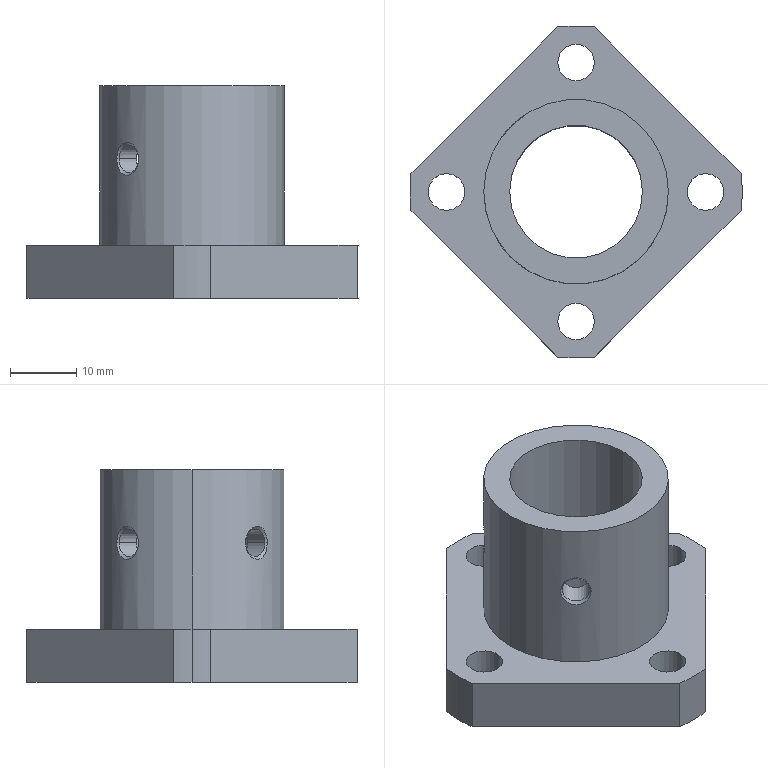Part | SolidWorks | features BaseBody 1 | 1 solid | 32 faces | box 50 x 50 x 32 mm | volume 15595 mm3 | cylinder 21 | plane 7 | cone 4 | commonest cylinder face diameters 5.5 x8 50 x5 4.134 x4 20 x2 27.8 x2
STEP:
#1=CARTESIAN_POINT('',(-11.324,8.061,13.));
#2=VERTEX_POINT('',#1);
#3=CARTESIAN_POINT('',(-8.061,11.324,13.));
#4=VERTEX_POINT('',#3);
#5=CARTESIAN_POINT('',(-11.324,8.061,13.));
#6=CARTESIAN_POINT('',(-11.324,8.061,12.686));
#7=CARTESIAN_POINT('',(-11.291,8.108,12.369));
#8=CARTESIAN_POINT('',(-11.194,8.241,11.927));
#9=CARTESIAN_POINT('',(-11.153,8.296,11.784));
#10=CARTESIAN_POINT('',(-11.055,8.426,11.513));
#11=CARTESIAN_POINT('',(-10.998,8.5,11.386));
#12=CARTESIAN_POINT('',(-10.869,8.666,11.151));
#13=CARTESIAN_POINT('',(-10.795,8.757,11.042));
#14=CARTESIAN_POINT('',(-10.635,8.952,10.853));
#15=CARTESIAN_POINT('',(-10.547,9.055,10.772));
#16=CARTESIAN_POINT('',(-10.357,9.271,10.637));
#17=CARTESIAN_POINT('',(-10.257,9.382,10.586));
#18=CARTESIAN_POINT('',(-10.048,9.606,10.517));
#19=CARTESIAN_POINT('',(-9.936,9.721,10.5));
#20=CARTESIAN_POINT('',(-9.603,10.054,10.501));
#21=CARTESIAN_POINT('',(-9.371,10.27,10.574));
#22=CARTESIAN_POINT('',(-9.052,10.55,10.774));
#23=CARTESIAN_POINT('',(-8.948,10.638,10.857));
#24=CARTESIAN_POINT('',(-8.753,10.799,11.047));
#25=CARTESIAN_POINT('',(-8.663,10.87,11.154));
#26=CARTESIAN_POINT('',(-8.499,10.999,11.388));
#27=CARTESIAN_POINT('',(-8.424,11.057,11.517));
#28=CARTESIAN_POINT('',(-8.295,11.154,11.787));
#29=CARTESIAN_POINT('',(-8.24,11.194,11.928));
#30=CARTESIAN_POINT('',(-8.152,11.259,12.222));
#31=CARTESIAN_POINT('',(-8.117,11.284,12.377));
#32=CARTESIAN_POINT('',(-8.072,11.316,12.686));
#33=CARTESIAN_POINT('',(-8.061,11.324,12.843));
#34=CARTESIAN_POINT('',(-8.061,11.324,13.));
#35=B_SPLINE_CURVE_WITH_KNOTS('',3,(#5,#6,#7,#8,#9,#10,#11,#12,#13,#14,#15,#16,#17,#18,#19,#20,#21,#22,#23,#24,#25,#26,#27,#28,#29,#30,#31,#32,#33,#34),.UNSPECIFIED.,.F.,.F.,(4,2,2,2,2,2,2,2,2,2,2,2,2,2,4),(0.003537,0.004487,0.004962,0.005436,0.005911,0.006386,0.006861,0.007336,0.008285,0.00876,0.009235,0.009709,0.01018,0.01066,0.01113),.UNSPECIFIED.);
#36=EDGE_CURVE('',#2,#4,#35,.T.);
#37=ORIENTED_EDGE('',*,*,#36,.T.);
#38=CARTESIAN_POINT('',(-8.061,11.324,13.));
#39=CARTESIAN_POINT('',(-8.061,11.324,13.157));
#40=CARTESIAN_POINT('',(-8.073,11.316,13.317));
#41=CARTESIAN_POINT('',(-8.118,11.283,13.626));
#42=CARTESIAN_POINT('',(-8.152,11.259,13.777));
#43=CARTESIAN_POINT('',(-8.285,11.161,14.221));
#44=CARTESIAN_POINT('',(-8.417,11.064,14.495));
#45=CARTESIAN_POINT('',(-8.666,10.869,14.849));
#46=CARTESIAN_POINT('',(-8.756,10.796,14.956));
#47=CARTESIAN_POINT('',(-8.95,10.636,15.145));
#48=CARTESIAN_POINT('',(-9.054,10.547,15.228));
#49=CARTESIAN_POINT('',(-9.376,10.266,15.428));
#50=CARTESIAN_POINT('',(-9.607,10.051,15.5));
#51=CARTESIAN_POINT('',(-10.051,9.607,15.5));
#52=CARTESIAN_POINT('',(-10.269,9.372,15.427));
#53=CARTESIAN_POINT('',(-10.55,9.051,15.226));
#54=CARTESIAN_POINT('',(-10.637,8.949,15.144));
#55=CARTESIAN_POINT('',(-10.797,8.755,14.955));
#56=CARTESIAN_POINT('',(-10.871,8.663,14.846));
#57=CARTESIAN_POINT('',(-10.999,8.499,14.612));
#58=CARTESIAN_POINT('',(-11.056,8.425,14.486));
#59=CARTESIAN_POINT('',(-11.153,8.296,14.215));
#60=CARTESIAN_POINT('',(-11.194,8.24,14.071));
#61=CARTESIAN_POINT('',(-11.259,8.152,13.778));
#62=CARTESIAN_POINT('',(-11.283,8.118,13.626));
#63=CARTESIAN_POINT('',(-11.316,8.072,13.315));
#64=CARTESIAN_POINT('',(-11.324,8.061,13.157));
#65=CARTESIAN_POINT('',(-11.324,8.061,13.));
#66=B_SPLINE_CURVE_WITH_KNOTS('',3,(#38,#39,#40,#41,#42,#43,#44,#45,#46,#47,#48,#49,#50,#51,#52,#53,#54,#55,#56,#57,#58,#59,#60,#61,#62,#63,#64,#65),.UNSPECIFIED.,.F.,.F.,(4,2,2,2,2,2,2,2,2,2,2,2,2,4),(0.01113,0.01161,0.01208,0.01303,0.01351,0.01398,0.01493,0.01588,0.01635,0.01683,0.0173,0.01778,0.01825,0.01873),.UNSPECIFIED.);
#67=EDGE_CURVE('',#4,#2,#66,.T.);
#68=ORIENTED_EDGE('',*,*,#67,.T.);
#69=EDGE_LOOP('',(#37,#68));
#70=FACE_BOUND('',#69,.T.);
#71=CARTESIAN_POINT('',(-13.9,0.,24.));
#72=VERTEX_POINT('',#71);
#73=CARTESIAN_POINT('',(13.9,0.,24.));
#74=VERTEX_POINT('',#73);
#75=CARTESIAN_POINT('',(0.,0.,24.));
#76=DIRECTION('',(0.,0.,-1.));
#77=DIRECTION('',(-1.,0.,0.));
#78=AXIS2_PLACEMENT_3D('',#75,#76,#77);
#79=CIRCLE('',#78,13.9);
#80=EDGE_CURVE('',#72,#74,#79,.T.);
#81=ORIENTED_EDGE('',*,*,#80,.T.);
#82=CARTESIAN_POINT('',(13.9,0.,0.));
#83=VERTEX_POINT('',#82);
#84=CARTESIAN_POINT('',(13.9,0.,0.));
#85=DIRECTION('',(0.,0.,-1.));
#86=VECTOR('',#85,1000.);
#87=LINE('',#84,#86);
#88=EDGE_CURVE('',#74,#83,#87,.T.);
#89=ORIENTED_EDGE('',*,*,#88,.T.);
#90=CARTESIAN_POINT('',(-13.9,0.,0.));
#91=VERTEX_POINT('',#90);
#92=CARTESIAN_POINT('',(0.,0.,0.));
#93=DIRECTION('',(0.,0.,1.));
#94=DIRECTION('',(-1.,0.,0.));
#95=AXIS2_PLACEMENT_3D('',#92,#93,#94);
#96=CIRCLE('',#95,13.9);
#97=EDGE_CURVE('',#83,#91,#96,.T.);
#98=ORIENTED_EDGE('',*,*,#97,.T.);
#99=CARTESIAN_POINT('',(-13.9,0.,0.));
#100=DIRECTION('',(0.,0.,-1.));
#101=VECTOR('',#100,1000.);
#102=LINE('',#99,#101);
#103=EDGE_CURVE('',#72,#91,#102,.T.);
#104=ORIENTED_EDGE('',*,*,#103,.F.);
#105=EDGE_LOOP('',(#81,#89,#98,#104));
#106=FACE_OUTER_BOUND('',#105,.T.);
#107=CARTESIAN_POINT('',(0.,0.,0.));
#108=DIRECTION('',(0.,0.,-1.));
#109=DIRECTION('',(-1.,0.,0.));
#110=AXIS2_PLACEMENT_3D('',#107,#108,#109);
#111=CYLINDRICAL_SURFACE('',#110,13.9);
#112=ADVANCED_FACE('',(#70,#106),#111,.T.);
#113=CARTESIAN_POINT('',(-25.,0.,0.));
#114=VERTEX_POINT('',#113);
#115=CARTESIAN_POINT('',(-24.851,-2.726,0.));
#116=VERTEX_POINT('',#115);
#117=CARTESIAN_POINT('',(0.,0.,0.));
#118=DIRECTION('',(0.,0.,1.));
#119=DIRECTION('',(-1.,0.,0.));
#120=AXIS2_PLACEMENT_3D('',#117,#118,#119);
#121=CIRCLE('',#120,25.);
#122=EDGE_CURVE('',#114,#116,#121,.T.);
#123=ORIENTED_EDGE('',*,*,#122,.F.);
#124=CARTESIAN_POINT('',(-25.,0.,-8.));
#125=VERTEX_POINT('',#124);
#126=CARTESIAN_POINT('',(-25.,0.,0.));
#127=DIRECTION('',(0.,0.,-1.));
#128=VECTOR('',#127,1000.);
#129=LINE('',#126,#128);
#130=EDGE_CURVE('',#114,#125,#129,.T.);
#131=ORIENTED_EDGE('',*,*,#130,.T.);
#132=CARTESIAN_POINT('',(-24.851,-2.726,-8.));
#133=VERTEX_POINT('',#132);
#134=CARTESIAN_POINT('',(0.,0.,-8.));
#135=DIRECTION('',(0.,0.,1.));
#136=DIRECTION('',(-1.,0.,0.));
#137=AXIS2_PLACEMENT_3D('',#134,#135,#136);
#138=CIRCLE('',#137,25.);
#139=EDGE_CURVE('',#125,#133,#138,.T.);
#140=ORIENTED_EDGE('',*,*,#139,.T.);
#141=CARTESIAN_POINT('',(-24.851,-2.726,-8.));
#142=DIRECTION('',(0.,0.,-1.));
#143=VECTOR('',#142,1000.);
#144=LINE('',#141,#143);
#145=EDGE_CURVE('',#116,#133,#144,.T.);
#146=ORIENTED_EDGE('',*,*,#145,.F.);
#147=EDGE_LOOP('',(#123,#131,#140,#146));
#148=FACE_OUTER_BOUND('',#147,.T.);
#149=CARTESIAN_POINT('',(0.,0.,0.));
#150=DIRECTION('',(0.,0.,-1.));
#151=DIRECTION('',(-1.,0.,0.));
#152=AXIS2_PLACEMENT_3D('',#149,#150,#151);
#153=CYLINDRICAL_SURFACE('',#152,25.);
#154=ADVANCED_FACE('',(#148),#153,.T.);
#155=CARTESIAN_POINT('',(-16.75,0.,0.));
#156=VERTEX_POINT('',#155);
#157=CARTESIAN_POINT('',(-22.25,0.,0.));
#158=VERTEX_POINT('',#157);
#159=CARTESIAN_POINT('',(-19.5,0.,0.));
#160=DIRECTION('',(0.,0.,-1.));
#161=DIRECTION('',(-1.,0.,0.));
#162=AXIS2_PLACEMENT_3D('',#159,#160,#161);
#163=CIRCLE('',#162,2.75);
#164=EDGE_CURVE('',#156,#158,#163,.T.);
#165=ORIENTED_EDGE('',*,*,#164,.F.);
#166=CARTESIAN_POINT('',(-16.75,0.,-8.));
#167=VERTEX_POINT('',#166);
#168=CARTESIAN_POINT('',(-16.75,0.,-8.));
#169=DIRECTION('',(0.,0.,-1.));
#170=VECTOR('',#169,1000.);
#171=LINE('',#168,#170);
#172=EDGE_CURVE('',#156,#167,#171,.T.);
#173=ORIENTED_EDGE('',*,*,#172,.T.);
#174=CARTESIAN_POINT('',(-22.25,0.,-8.));
#175=VERTEX_POINT('',#174);
#176=CARTESIAN_POINT('',(-19.5,0.,-8.));
#177=DIRECTION('',(0.,0.,1.));
#178=DIRECTION('',(-1.,0.,0.));
#179=AXIS2_PLACEMENT_3D('',#176,#177,#178);
#180=CIRCLE('',#179,2.75);
#181=EDGE_CURVE('',#175,#167,#180,.T.);
#182=ORIENTED_EDGE('',*,*,#181,.F.);
#183=CARTESIAN_POINT('',(-22.25,0.,-8.));
#184=DIRECTION('',(0.,0.,-1.));
#185=VECTOR('',#184,1000.);
#186=LINE('',#183,#185);
#187=EDGE_CURVE('',#158,#175,#186,.T.);
#188=ORIENTED_EDGE('',*,*,#187,.F.);
#189=EDGE_LOOP('',(#165,#173,#182,#188));
#190=FACE_OUTER_BOUND('',#189,.T.);
#191=CARTESIAN_POINT('',(-19.5,0.,-8.));
#192=DIRECTION('',(0.,0.,-1.));
#193=DIRECTION('',(-1.,0.,0.));
#194=AXIS2_PLACEMENT_3D('',#191,#192,#193);
#195=CYLINDRICAL_SURFACE('',#194,2.75);
#196=ADVANCED_FACE('',(#190),#195,.F.);
#197=CARTESIAN_POINT('',(2.75,-19.5,0.));
#198=VERTEX_POINT('',#197);
#199=CARTESIAN_POINT('',(-2.75,-19.5,0.));
#200=VERTEX_POINT('',#199);
#201=CARTESIAN_POINT('',(0.,-19.5,0.));
#202=DIRECTION('',(0.,0.,-1.));
#203=DIRECTION('',(-1.,0.,0.));
#204=AXIS2_PLACEMENT_3D('',#201,#202,#203);
#205=CIRCLE('',#204,2.75);
#206=EDGE_CURVE('',#198,#200,#205,.T.);
#207=ORIENTED_EDGE('',*,*,#206,.F.);
#208=CARTESIAN_POINT('',(2.75,-19.5,-8.));
#209=VERTEX_POINT('',#208);
#210=CARTESIAN_POINT('',(2.75,-19.5,-8.));
#211=DIRECTION('',(0.,0.,-1.));
#212=VECTOR('',#211,1000.);
#213=LINE('',#210,#212);
#214=EDGE_CURVE('',#198,#209,#213,.T.);
#215=ORIENTED_EDGE('',*,*,#214,.T.);
#216=CARTESIAN_POINT('',(-2.75,-19.5,-8.));
#217=VERTEX_POINT('',#216);
#218=CARTESIAN_POINT('',(0.,-19.5,-8.));
#219=DIRECTION('',(0.,0.,1.));
#220=DIRECTION('',(-1.,0.,0.));
#221=AXIS2_PLACEMENT_3D('',#218,#219,#220);
#222=CIRCLE('',#221,2.75);
#223=EDGE_CURVE('',#217,#209,#222,.T.);
#224=ORIENTED_EDGE('',*,*,#223,.F.);
#225=CARTESIAN_POINT('',(-2.75,-19.5,-8.));
#226=DIRECTION('',(0.,0.,-1.));
#227=VECTOR('',#226,1000.);
#228=LINE('',#225,#227);
#229=EDGE_CURVE('',#200,#217,#228,.T.);
#230=ORIENTED_EDGE('',*,*,#229,.F.);
#231=EDGE_LOOP('',(#207,#215,#224,#230));
#232=FACE_OUTER_BOUND('',#231,.T.);
#233=CARTESIAN_POINT('',(0.,-19.5,-8.));
#234=DIRECTION('',(0.,0.,-1.));
#235=DIRECTION('',(-1.,0.,0.));
#236=AXIS2_PLACEMENT_3D('',#233,#234,#235);
#237=CYLINDRICAL_SURFACE('',#236,2.75);
#238=ADVANCED_FACE('',(#232),#237,.F.);
#239=CARTESIAN_POINT('',(22.25,0.,0.));
#240=VERTEX_POINT('',#239);
#241=CARTESIAN_POINT('',(16.75,0.,0.));
#242=VERTEX_POINT('',#241);
#243=CARTESIAN_POINT('',(19.5,0.,0.));
#244=DIRECTION('',(0.,0.,-1.));
#245=DIRECTION('',(-1.,0.,0.));
#246=AXIS2_PLACEMENT_3D('',#243,#244,#245);
#247=CIRCLE('',#246,2.75);
#248=EDGE_CURVE('',#240,#242,#247,.T.);
#249=ORIENTED_EDGE('',*,*,#248,.F.);
#250=CARTESIAN_POINT('',(22.25,0.,-8.));
#251=VERTEX_POINT('',#250);
#252=CARTESIAN_POINT('',(22.25,0.,-8.));
#253=DIRECTION('',(0.,0.,-1.));
#254=VECTOR('',#253,1000.);
#255=LINE('',#252,#254);
#256=EDGE_CURVE('',#240,#251,#255,.T.);
#257=ORIENTED_EDGE('',*,*,#256,.T.);
#258=CARTESIAN_POINT('',(16.75,0.,-8.));
#259=VERTEX_POINT('',#258);
#260=CARTESIAN_POINT('',(19.5,0.,-8.));
#261=DIRECTION('',(0.,0.,1.));
#262=DIRECTION('',(-1.,0.,0.));
#263=AXIS2_PLACEMENT_3D('',#260,#261,#262);
#264=CIRCLE('',#263,2.75);
#265=EDGE_CURVE('',#259,#251,#264,.T.);
#266=ORIENTED_EDGE('',*,*,#265,.F.);
#267=CARTESIAN_POINT('',(16.75,0.,-8.));
#268=DIRECTION('',(0.,0.,-1.));
#269=VECTOR('',#268,1000.);
#270=LINE('',#267,#269);
#271=EDGE_CURVE('',#242,#259,#270,.T.);
#272=ORIENTED_EDGE('',*,*,#271,.F.);
#273=EDGE_LOOP('',(#249,#257,#266,#272));
#274=FACE_OUTER_BOUND('',#273,.T.);
#275=CARTESIAN_POINT('',(19.5,0.,-8.));
#276=DIRECTION('',(0.,0.,-1.));
#277=DIRECTION('',(-1.,0.,0.));
#278=AXIS2_PLACEMENT_3D('',#275,#276,#277);
#279=CYLINDRICAL_SURFACE('',#278,2.75);
#280=ADVANCED_FACE('',(#274),#279,.F.);
#281=CARTESIAN_POINT('',(2.75,19.5,0.));
#282=VERTEX_POINT('',#281);
#283=CARTESIAN_POINT('',(-2.75,19.5,0.));
#284=VERTEX_POINT('',#283);
#285=CARTESIAN_POINT('',(0.,19.5,0.));
#286=DIRECTION('',(0.,0.,-1.));
#287=DIRECTION('',(-1.,0.,0.));
#288=AXIS2_PLACEMENT_3D('',#285,#286,#287);
#289=CIRCLE('',#288,2.75);
#290=EDGE_CURVE('',#282,#284,#289,.T.);
#291=ORIENTED_EDGE('',*,*,#290,.F.);
#292=CARTESIAN_POINT('',(2.75,19.5,-8.));
#293=VERTEX_POINT('',#292);
#294=CARTESIAN_POINT('',(2.75,19.5,-8.));
#295=DIRECTION('',(0.,0.,-1.));
#296=VECTOR('',#295,1000.);
#297=LINE('',#294,#296);
#298=EDGE_CURVE('',#282,#293,#297,.T.);
#299=ORIENTED_EDGE('',*,*,#298,.T.);
#300=CARTESIAN_POINT('',(-2.75,19.5,-8.));
#301=VERTEX_POINT('',#300);
#302=CARTESIAN_POINT('',(0.,19.5,-8.));
#303=DIRECTION('',(0.,0.,1.));
#304=DIRECTION('',(-1.,0.,0.));
#305=AXIS2_PLACEMENT_3D('',#302,#303,#304);
#306=CIRCLE('',#305,2.75);
#307=EDGE_CURVE('',#301,#293,#306,.T.);
#308=ORIENTED_EDGE('',*,*,#307,.F.);
#309=CARTESIAN_POINT('',(-2.75,19.5,-8.));
#310=DIRECTION('',(0.,0.,-1.));
#311=VECTOR('',#310,1000.);
#312=LINE('',#309,#311);
#313=EDGE_CURVE('',#284,#301,#312,.T.);
#314=ORIENTED_EDGE('',*,*,#313,.F.);
#315=EDGE_LOOP('',(#291,#299,#308,#314));
#316=FACE_OUTER_BOUND('',#315,.T.);
#317=CARTESIAN_POINT('',(0.,19.5,-8.));
#318=DIRECTION('',(0.,0.,-1.));
#319=DIRECTION('',(-1.,0.,0.));
#320=AXIS2_PLACEMENT_3D('',#317,#318,#319);
#321=CYLINDRICAL_SURFACE('',#320,2.75);
#322=ADVANCED_FACE('',(#316),#321,.F.);
#323=CARTESIAN_POINT('',(-5.457,-8.38,13.));
#324=VERTEX_POINT('',#323);
#325=CARTESIAN_POINT('',(-8.38,-5.457,13.));
#326=VERTEX_POINT('',#325);
#327=CARTESIAN_POINT('',(-5.457,-8.38,13.));
#328=CARTESIAN_POINT('',(-5.457,-8.38,12.863));
#329=CARTESIAN_POINT('',(-5.468,-8.372,12.728));
#330=CARTESIAN_POINT('',(-5.513,-8.343,12.464));
#331=CARTESIAN_POINT('',(-5.547,-8.321,12.333));
#332=CARTESIAN_POINT('',(-5.635,-8.261,12.082));
#333=CARTESIAN_POINT('',(-5.688,-8.225,11.964));
#334=CARTESIAN_POINT('',(-5.813,-8.137,11.74));
#335=CARTESIAN_POINT('',(-5.884,-8.086,11.634));
#336=CARTESIAN_POINT('',(-6.039,-7.971,11.443));
#337=CARTESIAN_POINT('',(-6.122,-7.908,11.358));
#338=CARTESIAN_POINT('',(-6.3,-7.767,11.207));
#339=CARTESIAN_POINT('',(-6.393,-7.69,11.143));
#340=CARTESIAN_POINT('',(-6.678,-7.448,10.988));
#341=CARTESIAN_POINT('',(-6.879,-7.263,10.933));
#342=CARTESIAN_POINT('',(-7.166,-6.976,10.933));
#343=CARTESIAN_POINT('',(-7.261,-6.877,10.946));
#344=CARTESIAN_POINT('',(-7.441,-6.682,10.999));
#345=CARTESIAN_POINT('',(-7.527,-6.585,11.038));
#346=CARTESIAN_POINT('',(-7.689,-6.394,11.142));
#347=CARTESIAN_POINT('',(-7.766,-6.301,11.207));
#348=CARTESIAN_POINT('',(-7.906,-6.124,11.356));
#349=CARTESIAN_POINT('',(-7.97,-6.041,11.441));
#350=CARTESIAN_POINT('',(-8.086,-5.884,11.634));
#351=CARTESIAN_POINT('',(-8.137,-5.814,11.738));
#352=CARTESIAN_POINT('',(-8.225,-5.689,11.963));
#353=CARTESIAN_POINT('',(-8.262,-5.634,12.084));
#354=CARTESIAN_POINT('',(-8.35,-5.504,12.457));
#355=CARTESIAN_POINT('',(-8.38,-5.457,12.73));
#356=CARTESIAN_POINT('',(-8.38,-5.457,13.));
#357=B_SPLINE_CURVE_WITH_KNOTS('',3,(#327,#328,#329,#330,#331,#332,#333,#334,#335,#336,#337,#338,#339,#340,#341,#342,#343,#344,#345,#346,#347,#348,#349,#350,#351,#352,#353,#354,#355,#356),.UNSPECIFIED.,.F.,.F.,(4,2,2,2,2,2,2,2,2,2,2,2,2,2,4),(0.008144,0.008552,0.008959,0.009366,0.009774,0.01018,0.01059,0.0114,0.01181,0.01222,0.01262,0.01303,0.01344,0.01385,0.01466),.UNSPECIFIED.);
#358=EDGE_CURVE('',#324,#326,#357,.T.);
#359=ORIENTED_EDGE('',*,*,#358,.F.);
#360=CARTESIAN_POINT('',(-8.38,-5.457,13.));
#361=CARTESIAN_POINT('',(-8.38,-5.457,13.135));
#362=CARTESIAN_POINT('',(-8.372,-5.468,13.272));
#363=CARTESIAN_POINT('',(-8.343,-5.514,13.538));
#364=CARTESIAN_POINT('',(-8.321,-5.547,13.667));
#365=CARTESIAN_POINT('',(-8.262,-5.635,13.917));
#366=CARTESIAN_POINT('',(-8.224,-5.689,14.038));
#367=CARTESIAN_POINT('',(-8.137,-5.813,14.261));
#368=CARTESIAN_POINT('',(-8.087,-5.884,14.365));
#369=CARTESIAN_POINT('',(-7.913,-6.117,14.653));
#370=CARTESIAN_POINT('',(-7.772,-6.297,14.805));
#371=CARTESIAN_POINT('',(-7.527,-6.585,14.961));
#372=CARTESIAN_POINT('',(-7.441,-6.682,15.001));
#373=CARTESIAN_POINT('',(-7.261,-6.877,15.053));
#374=CARTESIAN_POINT('',(-7.166,-6.976,15.067));
#375=CARTESIAN_POINT('',(-6.975,-7.167,15.067));
#376=CARTESIAN_POINT('',(-6.878,-7.26,15.054));
#377=CARTESIAN_POINT('',(-6.682,-7.441,15.001));
#378=CARTESIAN_POINT('',(-6.583,-7.528,14.961));
#379=CARTESIAN_POINT('',(-6.299,-7.771,14.806));
#380=CARTESIAN_POINT('',(-6.116,-7.914,14.652));
#381=CARTESIAN_POINT('',(-5.885,-8.086,14.367));
#382=CARTESIAN_POINT('',(-5.813,-8.137,14.261));
#383=CARTESIAN_POINT('',(-5.688,-8.225,14.036));
#384=CARTESIAN_POINT('',(-5.635,-8.261,13.918));
#385=CARTESIAN_POINT('',(-5.547,-8.32,13.668));
#386=CARTESIAN_POINT('',(-5.513,-8.343,13.536));
#387=CARTESIAN_POINT('',(-5.468,-8.372,13.271));
#388=CARTESIAN_POINT('',(-5.457,-8.38,13.137));
#389=CARTESIAN_POINT('',(-5.457,-8.38,13.));
#390=B_SPLINE_CURVE_WITH_KNOTS('',3,(#360,#361,#362,#363,#364,#365,#366,#367,#368,#369,#370,#371,#372,#373,#374,#375,#376,#377,#378,#379,#380,#381,#382,#383,#384,#385,#386,#387,#388,#389),.UNSPECIFIED.,.F.,.F.,(4,2,2,2,2,2,2,2,2,2,2,2,2,2,4),(0.001626,0.002033,0.002441,0.002848,0.003255,0.00407,0.004478,0.004885,0.005293,0.0057,0.006515,0.006922,0.00733,0.007737,0.008144),.UNSPECIFIED.);
#391=EDGE_CURVE('',#326,#324,#390,.T.);
#392=ORIENTED_EDGE('',*,*,#391,.F.);
#393=EDGE_LOOP('',(#359,#392));
#394=FACE_BOUND('',#393,.T.);
#395=CARTESIAN_POINT('',(10.,0.,24.));
#396=VERTEX_POINT('',#395);
#397=CARTESIAN_POINT('',(-10.,0.,24.));
#398=VERTEX_POINT('',#397);
#399=CARTESIAN_POINT('',(0.,0.,24.));
#400=DIRECTION('',(0.,0.,-1.));
#401=DIRECTION('',(-1.,0.,0.));
#402=AXIS2_PLACEMENT_3D('',#399,#400,#401);
#403=CIRCLE('',#402,10.);
#404=EDGE_CURVE('',#396,#398,#403,.T.);
#405=ORIENTED_EDGE('',*,*,#404,.F.);
#406=CARTESIAN_POINT('',(10.,0.,-8.));
#407=VERTEX_POINT('',#406);
#408=CARTESIAN_POINT('',(10.,0.,0.));
#409=DIRECTION('',(0.,0.,-1.));
#410=VECTOR('',#409,1000.);
#411=LINE('',#408,#410);
#412=EDGE_CURVE('',#396,#407,#411,.T.);
#413=ORIENTED_EDGE('',*,*,#412,.T.);
#414=CARTESIAN_POINT('',(-10.,0.,-8.));
#415=VERTEX_POINT('',#414);
#416=CARTESIAN_POINT('',(0.,0.,-8.));
#417=DIRECTION('',(0.,0.,1.));
#418=DIRECTION('',(-1.,0.,0.));
#419=AXIS2_PLACEMENT_3D('',#416,#417,#418);
#420=CIRCLE('',#419,10.);
#421=EDGE_CURVE('',#415,#407,#420,.T.);
#422=ORIENTED_EDGE('',*,*,#421,.F.);
#423=CARTESIAN_POINT('',(-10.,0.,0.));
#424=DIRECTION('',(0.,0.,-1.));
#425=VECTOR('',#424,1000.);
#426=LINE('',#423,#425);
#427=EDGE_CURVE('',#398,#415,#426,.T.);
#428=ORIENTED_EDGE('',*,*,#427,.F.);
#429=EDGE_LOOP('',(#405,#413,#422,#428));
#430=FACE_OUTER_BOUND('',#429,.T.);
#431=CARTESIAN_POINT('',(0.,0.,0.));
#432=DIRECTION('',(0.,0.,-1.));
#433=DIRECTION('',(-1.,0.,0.));
#434=AXIS2_PLACEMENT_3D('',#431,#432,#433);
#435=CYLINDRICAL_SURFACE('',#434,10.);
#436=ADVANCED_FACE('',(#394,#430),#435,.F.);
#437=ORIENTED_EDGE('',*,*,#358,.T.);
#438=CARTESIAN_POINT('',(-10.984,-8.061,13.));
#439=VERTEX_POINT('',#438);
#440=CARTESIAN_POINT('',(-11.29,-8.367,13.));
#441=DIRECTION('',(-0.7071,-0.7071,0.));
#442=VECTOR('',#441,1000.);
#443=LINE('',#440,#442);
#444=EDGE_CURVE('',#326,#439,#443,.T.);
#445=ORIENTED_EDGE('',*,*,#444,.T.);
#446=CARTESIAN_POINT('',(-8.061,-10.984,13.));
#447=VERTEX_POINT('',#446);
#448=CARTESIAN_POINT('',(-9.523,-9.523,13.));
#449=DIRECTION('',(0.7071,0.7071,0.));
#450=DIRECTION('',(0.7071,-0.7071,0.));
#451=AXIS2_PLACEMENT_3D('',#448,#449,#450);
#452=CIRCLE('',#451,2.067);
#453=EDGE_CURVE('',#447,#439,#452,.T.);
#454=ORIENTED_EDGE('',*,*,#453,.F.);
#455=CARTESIAN_POINT('',(-8.367,-11.29,13.));
#456=DIRECTION('',(-0.7071,-0.7071,0.));
#457=VECTOR('',#456,1000.);
#458=LINE('',#455,#457);
#459=EDGE_CURVE('',#324,#447,#458,.T.);
#460=ORIENTED_EDGE('',*,*,#459,.F.);
#461=EDGE_LOOP('',(#437,#445,#454,#460));
#462=FACE_OUTER_BOUND('',#461,.T.);
#463=CARTESIAN_POINT('',(-9.829,-9.829,13.));
#464=DIRECTION('',(-0.7071,-0.7071,0.));
#465=DIRECTION('',(0.7071,-0.7071,0.));
#466=AXIS2_PLACEMENT_3D('',#463,#464,#465);
#467=CYLINDRICAL_SURFACE('',#466,2.067);
#468=ADVANCED_FACE('',(#462),#467,.F.);
#469=ORIENTED_EDGE('',*,*,#453,.T.);
#470=CARTESIAN_POINT('',(-11.324,-8.061,13.));
#471=VERTEX_POINT('',#470);
#472=CARTESIAN_POINT('',(-11.641,-8.061,13.));
#473=DIRECTION('',(-1.,0.,0.));
#474=VECTOR('',#473,1000.);
#475=LINE('',#472,#474);
#476=EDGE_CURVE('',#439,#471,#475,.T.);
#477=ORIENTED_EDGE('',*,*,#476,.T.);
#478=CARTESIAN_POINT('',(-8.061,-11.324,13.));
#479=VERTEX_POINT('',#478);
#480=CARTESIAN_POINT('',(-8.061,-11.324,13.));
#481=CARTESIAN_POINT('',(-8.061,-11.324,12.843));
#482=CARTESIAN_POINT('',(-8.072,-11.316,12.686));
#483=CARTESIAN_POINT('',(-8.118,-11.283,12.376));
#484=CARTESIAN_POINT('',(-8.152,-11.259,12.222));
#485=CARTESIAN_POINT('',(-8.285,-11.161,11.78));
#486=CARTESIAN_POINT('',(-8.418,-11.063,11.503));
#487=CARTESIAN_POINT('',(-8.665,-10.869,11.151));
#488=CARTESIAN_POINT('',(-8.757,-10.795,11.043));
#489=CARTESIAN_POINT('',(-8.952,-10.634,10.853));
#490=CARTESIAN_POINT('',(-9.054,-10.547,10.772));
#491=CARTESIAN_POINT('',(-9.27,-10.358,10.638));
#492=CARTESIAN_POINT('',(-9.382,-10.257,10.586));
#493=CARTESIAN_POINT('',(-9.606,-10.048,10.517));
#494=CARTESIAN_POINT('',(-9.72,-9.937,10.5));
#495=CARTESIAN_POINT('',(-9.944,-9.714,10.5));
#496=CARTESIAN_POINT('',(-10.052,-9.602,10.518));
#497=CARTESIAN_POINT('',(-10.262,-9.377,10.588));
#498=CARTESIAN_POINT('',(-10.363,-9.265,10.641));
#499=CARTESIAN_POINT('',(-10.643,-8.945,10.841));
#500=CARTESIAN_POINT('',(-10.806,-8.745,11.037));
#501=CARTESIAN_POINT('',(-11.064,-8.417,11.504));
#502=CARTESIAN_POINT('',(-11.162,-8.284,11.782));
#503=CARTESIAN_POINT('',(-11.291,-8.108,12.369));
#504=CARTESIAN_POINT('',(-11.324,-8.061,12.686));
#505=CARTESIAN_POINT('',(-11.324,-8.061,13.));
#506=B_SPLINE_CURVE_WITH_KNOTS('',3,(#480,#481,#482,#483,#484,#485,#486,#487,#488,#489,#490,#491,#492,#493,#494,#495,#496,#497,#498,#499,#500,#501,#502,#503,#504,#505),.UNSPECIFIED.,.F.,.F.,(4,2,2,2,2,2,2,2,2,2,2,2,4),(0.001887,0.002359,0.002831,0.003775,0.004246,0.004718,0.00519,0.005662,0.006134,0.006605,0.007549,0.008493,0.009436),.UNSPECIFIED.);
#507=EDGE_CURVE('',#479,#471,#506,.T.);
#508=ORIENTED_EDGE('',*,*,#507,.F.);
#509=CARTESIAN_POINT('',(-8.061,-11.641,13.));
#510=DIRECTION('',(0.,-1.,0.));
#511=VECTOR('',#510,1000.);
#512=LINE('',#509,#511);
#513=EDGE_CURVE('',#447,#479,#512,.T.);
#514=ORIENTED_EDGE('',*,*,#513,.F.);
#515=EDGE_LOOP('',(#469,#477,#508,#514));
#516=FACE_OUTER_BOUND('',#515,.T.);
#517=CARTESIAN_POINT('',(-9.851,-9.851,13.));
#518=DIRECTION('',(-0.7071,-0.7071,0.));
#519=DIRECTION('',(0.7071,-0.7071,0.));
#520=AXIS2_PLACEMENT_3D('',#517,#518,#519);
#521=CONICAL_SURFACE('',#520,2.532,0.7854);
#522=ADVANCED_FACE('',(#516),#521,.F.);
#523=CARTESIAN_POINT('',(-8.38,5.457,13.));
#524=VERTEX_POINT('',#523);
#525=CARTESIAN_POINT('',(-5.457,8.38,13.));
#526=VERTEX_POINT('',#525);
#527=CARTESIAN_POINT('',(-8.38,5.457,13.));
#528=CARTESIAN_POINT('',(-8.38,5.457,12.863));
#529=CARTESIAN_POINT('',(-8.372,5.468,12.728));
#530=CARTESIAN_POINT('',(-8.343,5.513,12.464));
#531=CARTESIAN_POINT('',(-8.321,5.547,12.333));
#532=CARTESIAN_POINT('',(-8.261,5.635,12.082));
#533=CARTESIAN_POINT('',(-8.225,5.688,11.964));
#534=CARTESIAN_POINT('',(-8.137,5.813,11.74));
#535=CARTESIAN_POINT('',(-8.086,5.884,11.634));
#536=CARTESIAN_POINT('',(-7.971,6.039,11.443));
#537=CARTESIAN_POINT('',(-7.908,6.122,11.358));
#538=CARTESIAN_POINT('',(-7.767,6.3,11.207));
#539=CARTESIAN_POINT('',(-7.69,6.393,11.143));
#540=CARTESIAN_POINT('',(-7.448,6.678,10.988));
#541=CARTESIAN_POINT('',(-7.263,6.879,10.933));
#542=CARTESIAN_POINT('',(-6.976,7.166,10.933));
#543=CARTESIAN_POINT('',(-6.877,7.261,10.946));
#544=CARTESIAN_POINT('',(-6.682,7.441,10.999));
#545=CARTESIAN_POINT('',(-6.585,7.527,11.038));
#546=CARTESIAN_POINT('',(-6.394,7.689,11.142));
#547=CARTESIAN_POINT('',(-6.301,7.766,11.207));
#548=CARTESIAN_POINT('',(-6.124,7.906,11.356));
#549=CARTESIAN_POINT('',(-6.041,7.97,11.441));
#550=CARTESIAN_POINT('',(-5.884,8.086,11.634));
#551=CARTESIAN_POINT('',(-5.814,8.137,11.738));
#552=CARTESIAN_POINT('',(-5.689,8.225,11.963));
#553=CARTESIAN_POINT('',(-5.634,8.262,12.084));
#554=CARTESIAN_POINT('',(-5.504,8.35,12.457));
#555=CARTESIAN_POINT('',(-5.457,8.38,12.73));
#556=CARTESIAN_POINT('',(-5.457,8.38,13.));
#557=B_SPLINE_CURVE_WITH_KNOTS('',3,(#527,#528,#529,#530,#531,#532,#533,#534,#535,#536,#537,#538,#539,#540,#541,#542,#543,#544,#545,#546,#547,#548,#549,#550,#551,#552,#553,#554,#555,#556),.UNSPECIFIED.,.F.,.F.,(4,2,2,2,2,2,2,2,2,2,2,2,2,2,4),(0.008144,0.008552,0.008959,0.009366,0.009774,0.01018,0.01059,0.0114,0.01181,0.01222,0.01262,0.01303,0.01344,0.01385,0.01466),.UNSPECIFIED.);
#558=EDGE_CURVE('',#524,#526,#557,.T.);
#559=ORIENTED_EDGE('',*,*,#558,.T.);
#560=CARTESIAN_POINT('',(-8.061,10.984,13.));
#561=VERTEX_POINT('',#560);
#562=CARTESIAN_POINT('',(-8.367,11.29,13.));
#563=DIRECTION('',(-0.7071,0.7071,0.));
#564=VECTOR('',#563,1000.);
#565=LINE('',#562,#564);
#566=EDGE_CURVE('',#526,#561,#565,.T.);
#567=ORIENTED_EDGE('',*,*,#566,.T.);
#568=CARTESIAN_POINT('',(-10.984,8.061,13.));
#569=VERTEX_POINT('',#568);
#570=CARTESIAN_POINT('',(-9.523,9.523,13.));
#571=DIRECTION('',(0.7071,-0.7071,0.));
#572=DIRECTION('',(-0.7071,-0.7071,0.));
#573=AXIS2_PLACEMENT_3D('',#570,#571,#572);
#574=CIRCLE('',#573,2.067);
#575=EDGE_CURVE('',#569,#561,#574,.T.);
#576=ORIENTED_EDGE('',*,*,#575,.F.);
#577=CARTESIAN_POINT('',(-11.29,8.367,13.));
#578=DIRECTION('',(-0.7071,0.7071,0.));
#579=VECTOR('',#578,1000.);
#580=LINE('',#577,#579);
#581=EDGE_CURVE('',#524,#569,#580,.T.);
#582=ORIENTED_EDGE('',*,*,#581,.F.);
#583=EDGE_LOOP('',(#559,#567,#576,#582));
#584=FACE_OUTER_BOUND('',#583,.T.);
#585=CARTESIAN_POINT('',(-9.829,9.829,13.));
#586=DIRECTION('',(-0.7071,0.7071,0.));
#587=DIRECTION('',(-0.7071,-0.7071,0.));
#588=AXIS2_PLACEMENT_3D('',#585,#586,#587);
#589=CYLINDRICAL_SURFACE('',#588,2.067);
#590=ADVANCED_FACE('',(#584),#589,.F.);
#591=ORIENTED_EDGE('',*,*,#575,.T.);
#592=CARTESIAN_POINT('',(-8.061,11.605,13.));
#593=DIRECTION('',(0.,1.,0.));
#594=VECTOR('',#593,1000.);
#595=LINE('',#592,#594);
#596=EDGE_CURVE('',#561,#4,#595,.T.);
#597=ORIENTED_EDGE('',*,*,#596,.T.);
#598=ORIENTED_EDGE('',*,*,#36,.F.);
#599=CARTESIAN_POINT('',(-11.605,8.061,13.));
#600=DIRECTION('',(-1.,0.,0.));
#601=VECTOR('',#600,1000.);
#602=LINE('',#599,#601);
#603=EDGE_CURVE('',#569,#2,#602,.T.);
#604=ORIENTED_EDGE('',*,*,#603,.F.);
#605=EDGE_LOOP('',(#591,#597,#598,#604));
#606=FACE_OUTER_BOUND('',#605,.T.);
#607=CARTESIAN_POINT('',(-9.833,9.833,13.));
#608=DIRECTION('',(-0.7071,0.7071,0.));
#609=DIRECTION('',(-0.7071,-0.7071,0.));
#610=AXIS2_PLACEMENT_3D('',#607,#608,#609);
#611=CONICAL_SURFACE('',#610,2.506,0.7854);
#612=ADVANCED_FACE('',(#606),#611,.F.);
#613=ORIENTED_EDGE('',*,*,#88,.F.);
#614=CARTESIAN_POINT('',(0.,0.,24.));
#615=DIRECTION('',(0.,0.,-1.));
#616=DIRECTION('',(-1.,0.,0.));
#617=AXIS2_PLACEMENT_3D('',#614,#615,#616);
#618=CIRCLE('',#617,13.9);
#619=EDGE_CURVE('',#74,#72,#618,.T.);
#620=ORIENTED_EDGE('',*,*,#619,.T.);
#621=ORIENTED_EDGE('',*,*,#103,.T.);
#622=CARTESIAN_POINT('',(0.,0.,0.));
#623=DIRECTION('',(0.,0.,1.));
#624=DIRECTION('',(-1.,0.,0.));
#625=AXIS2_PLACEMENT_3D('',#622,#623,#624);
#626=CIRCLE('',#625,13.9);
#627=EDGE_CURVE('',#91,#83,#626,.T.);
#628=ORIENTED_EDGE('',*,*,#627,.T.);
#629=EDGE_LOOP('',(#613,#620,#621,#628));
#630=FACE_OUTER_BOUND('',#629,.T.);
#631=ORIENTED_EDGE('',*,*,#507,.T.);
#632=CARTESIAN_POINT('',(-11.324,-8.061,13.));
#633=CARTESIAN_POINT('',(-11.324,-8.061,13.157));
#634=CARTESIAN_POINT('',(-11.316,-8.072,13.315));
#635=CARTESIAN_POINT('',(-11.283,-8.118,13.626));
#636=CARTESIAN_POINT('',(-11.259,-8.152,13.777));
#637=CARTESIAN_POINT('',(-11.194,-8.24,14.072));
#638=CARTESIAN_POINT('',(-11.153,-8.296,14.216));
#639=CARTESIAN_POINT('',(-11.056,-8.425,14.486));
#640=CARTESIAN_POINT('',(-10.999,-8.499,14.612));
#641=CARTESIAN_POINT('',(-10.804,-8.748,14.966));
#642=CARTESIAN_POINT('',(-10.642,-8.946,15.161));
#643=CARTESIAN_POINT('',(-10.359,-9.269,15.362));
#644=CARTESIAN_POINT('',(-10.26,-9.379,15.413));
#645=CARTESIAN_POINT('',(-10.05,-9.604,15.482));
#646=CARTESIAN_POINT('',(-9.939,-9.718,15.5));
#647=CARTESIAN_POINT('',(-9.718,-9.94,15.5));
#648=CARTESIAN_POINT('',(-9.604,-10.05,15.482));
#649=CARTESIAN_POINT('',(-9.379,-10.26,15.413));
#650=CARTESIAN_POINT('',(-9.269,-10.359,15.362));
#651=CARTESIAN_POINT('',(-9.055,-10.547,15.229));
#652=CARTESIAN_POINT('',(-8.95,-10.636,15.146));
#653=CARTESIAN_POINT('',(-8.756,-10.796,14.957));
#654=CARTESIAN_POINT('',(-8.666,-10.868,14.85));
#655=CARTESIAN_POINT('',(-8.5,-10.999,14.613));
#656=CARTESIAN_POINT('',(-8.426,-11.056,14.486));
#657=CARTESIAN_POINT('',(-8.296,-11.153,14.216));
#658=CARTESIAN_POINT('',(-8.241,-11.194,14.072));
#659=CARTESIAN_POINT('',(-8.152,-11.259,13.777));
#660=CARTESIAN_POINT('',(-8.118,-11.283,13.626));
#661=CARTESIAN_POINT('',(-8.073,-11.316,13.317));
#662=CARTESIAN_POINT('',(-8.061,-11.324,13.157));
#663=CARTESIAN_POINT('',(-8.061,-11.324,13.));
#664=B_SPLINE_CURVE_WITH_KNOTS('',3,(#632,#633,#634,#635,#636,#637,#638,#639,#640,#641,#642,#643,#644,#645,#646,#647,#648,#649,#650,#651,#652,#653,#654,#655,#656,#657,#658,#659,#660,#661,#662,#663),.UNSPECIFIED.,.F.,.F.,(4,2,2,2,2,2,2,2,2,2,2,2,2,2,2,4),(0.009436,0.009908,0.01038,0.01085,0.01132,0.01227,0.01274,0.01321,0.01368,0.01415,0.01462,0.01509,0.01557,0.01604,0.01651,0.01698),.UNSPECIFIED.);
#665=EDGE_CURVE('',#471,#479,#664,.T.);
#666=ORIENTED_EDGE('',*,*,#665,.T.);
#667=EDGE_LOOP('',(#631,#666));
#668=FACE_BOUND('',#667,.T.);
#669=CARTESIAN_POINT('',(0.,0.,0.));
#670=DIRECTION('',(0.,0.,-1.));
#671=DIRECTION('',(-1.,0.,0.));
#672=AXIS2_PLACEMENT_3D('',#669,#670,#671);
#673=CYLINDRICAL_SURFACE('',#672,13.9);
#674=ADVANCED_FACE('',(#630,#668),#673,.T.);
#675=CARTESIAN_POINT('',(2.726,24.851,0.));
#676=VERTEX_POINT('',#675);
#677=CARTESIAN_POINT('',(-2.726,24.851,0.));
#678=VERTEX_POINT('',#677);
#679=CARTESIAN_POINT('',(0.,0.,0.));
#680=DIRECTION('',(0.,0.,1.));
#681=DIRECTION('',(-1.,0.,0.));
#682=AXIS2_PLACEMENT_3D('',#679,#680,#681);
#683=CIRCLE('',#682,25.);
#684=EDGE_CURVE('',#676,#678,#683,.T.);
#685=ORIENTED_EDGE('',*,*,#684,.T.);
#686=CARTESIAN_POINT('',(-24.851,2.726,0.));
#687=VERTEX_POINT('',#686);
#688=CARTESIAN_POINT('',(-2.726,24.851,0.));
#689=DIRECTION('',(-0.7071,-0.7071,0.));
#690=VECTOR('',#689,1000.);
#691=LINE('',#688,#690);
#692=EDGE_CURVE('',#678,#687,#691,.T.);
#693=ORIENTED_EDGE('',*,*,#692,.T.);
#694=CARTESIAN_POINT('',(0.,0.,0.));
#695=DIRECTION('',(0.,0.,1.));
#696=DIRECTION('',(-1.,0.,0.));
#697=AXIS2_PLACEMENT_3D('',#694,#695,#696);
#698=CIRCLE('',#697,25.);
#699=EDGE_CURVE('',#687,#114,#698,.T.);
#700=ORIENTED_EDGE('',*,*,#699,.T.);
#701=ORIENTED_EDGE('',*,*,#122,.T.);
#702=CARTESIAN_POINT('',(-2.726,-24.851,0.));
#703=VERTEX_POINT('',#702);
#704=CARTESIAN_POINT('',(-24.851,-2.726,0.));
#705=DIRECTION('',(0.7071,-0.7071,0.));
#706=VECTOR('',#705,1000.);
#707=LINE('',#704,#706);
#708=EDGE_CURVE('',#116,#703,#707,.T.);
#709=ORIENTED_EDGE('',*,*,#708,.T.);
#710=CARTESIAN_POINT('',(2.726,-24.851,0.));
#711=VERTEX_POINT('',#710);
#712=CARTESIAN_POINT('',(0.,0.,0.));
#713=DIRECTION('',(0.,0.,1.));
#714=DIRECTION('',(-1.,0.,0.));
#715=AXIS2_PLACEMENT_3D('',#712,#713,#714);
#716=CIRCLE('',#715,25.);
#717=EDGE_CURVE('',#703,#711,#716,.T.);
#718=ORIENTED_EDGE('',*,*,#717,.T.);
#719=CARTESIAN_POINT('',(24.851,-2.726,0.));
#720=VERTEX_POINT('',#719);
#721=CARTESIAN_POINT('',(2.726,-24.851,0.));
#722=DIRECTION('',(0.7071,0.7071,0.));
#723=VECTOR('',#722,1000.);
#724=LINE('',#721,#723);
#725=EDGE_CURVE('',#711,#720,#724,.T.);
#726=ORIENTED_EDGE('',*,*,#725,.T.);
#727=CARTESIAN_POINT('',(24.851,2.726,0.));
#728=VERTEX_POINT('',#727);
#729=CARTESIAN_POINT('',(0.,0.,0.));
#730=DIRECTION('',(0.,0.,1.));
#731=DIRECTION('',(-1.,0.,0.));
#732=AXIS2_PLACEMENT_3D('',#729,#730,#731);
#733=CIRCLE('',#732,25.);
#734=EDGE_CURVE('',#720,#728,#733,.T.);
#735=ORIENTED_EDGE('',*,*,#734,.T.);
#736=CARTESIAN_POINT('',(24.851,2.726,0.));
#737=DIRECTION('',(-0.7071,0.7071,0.));
#738=VECTOR('',#737,1000.);
#739=LINE('',#736,#738);
#740=EDGE_CURVE('',#728,#676,#739,.T.);
#741=ORIENTED_EDGE('',*,*,#740,.T.);
#742=EDGE_LOOP('',(#685,#693,#700,#701,#709,#718,#726,#735,#741));
#743=FACE_OUTER_BOUND('',#742,.T.);
#744=CARTESIAN_POINT('',(-19.5,0.,0.));
#745=DIRECTION('',(0.,0.,-1.));
#746=DIRECTION('',(-1.,0.,0.));
#747=AXIS2_PLACEMENT_3D('',#744,#745,#746);
#748=CIRCLE('',#747,2.75);
#749=EDGE_CURVE('',#158,#156,#748,.T.);
#750=ORIENTED_EDGE('',*,*,#749,.T.);
#751=ORIENTED_EDGE('',*,*,#164,.T.);
#752=EDGE_LOOP('',(#750,#751));
#753=FACE_BOUND('',#752,.T.);
#754=CARTESIAN_POINT('',(0.,-19.5,0.));
#755=DIRECTION('',(0.,0.,-1.));
#756=DIRECTION('',(-1.,0.,0.));
#757=AXIS2_PLACEMENT_3D('',#754,#755,#756);
#758=CIRCLE('',#757,2.75);
#759=EDGE_CURVE('',#200,#198,#758,.T.);
#760=ORIENTED_EDGE('',*,*,#759,.T.);
#761=ORIENTED_EDGE('',*,*,#206,.T.);
#762=EDGE_LOOP('',(#760,#761));
#763=FACE_BOUND('',#762,.T.);
#764=CARTESIAN_POINT('',(19.5,0.,0.));
#765=DIRECTION('',(0.,0.,-1.));
#766=DIRECTION('',(-1.,0.,0.));
#767=AXIS2_PLACEMENT_3D('',#764,#765,#766);
#768=CIRCLE('',#767,2.75);
#769=EDGE_CURVE('',#242,#240,#768,.T.);
#770=ORIENTED_EDGE('',*,*,#769,.T.);
#771=ORIENTED_EDGE('',*,*,#248,.T.);
#772=EDGE_LOOP('',(#770,#771));
#773=FACE_BOUND('',#772,.T.);
#774=CARTESIAN_POINT('',(0.,19.5,0.));
#775=DIRECTION('',(0.,0.,-1.));
#776=DIRECTION('',(-1.,0.,0.));
#777=AXIS2_PLACEMENT_3D('',#774,#775,#776);
#778=CIRCLE('',#777,2.75);
#779=EDGE_CURVE('',#284,#282,#778,.T.);
#780=ORIENTED_EDGE('',*,*,#779,.T.);
#781=ORIENTED_EDGE('',*,*,#290,.T.);
#782=EDGE_LOOP('',(#780,#781));
#783=FACE_BOUND('',#782,.T.);
#784=ORIENTED_EDGE('',*,*,#627,.F.);
#785=ORIENTED_EDGE('',*,*,#97,.F.);
#786=EDGE_LOOP('',(#784,#785));
#787=FACE_BOUND('',#786,.T.);
#788=CARTESIAN_POINT('',(0.,25.,0.));
#789=DIRECTION('',(0.,0.,1.));
#790=DIRECTION('',(1.,0.,0.));
#791=AXIS2_PLACEMENT_3D('',#788,#789,#790);
#792=PLANE('',#791);
#793=ADVANCED_FACE('',(#743,#753,#763,#773,#783,#787),#792,.T.);
#794=ORIENTED_EDGE('',*,*,#80,.F.);
#795=ORIENTED_EDGE('',*,*,#619,.F.);
#796=EDGE_LOOP('',(#794,#795));
#797=FACE_OUTER_BOUND('',#796,.T.);
#798=CARTESIAN_POINT('',(0.,0.,24.));
#799=DIRECTION('',(0.,0.,-1.));
#800=DIRECTION('',(-1.,0.,0.));
#801=AXIS2_PLACEMENT_3D('',#798,#799,#800);
#802=CIRCLE('',#801,10.);
#803=EDGE_CURVE('',#398,#396,#802,.T.);
#804=ORIENTED_EDGE('',*,*,#803,.T.);
#805=ORIENTED_EDGE('',*,*,#404,.T.);
#806=EDGE_LOOP('',(#804,#805));
#807=FACE_BOUND('',#806,.T.);
#808=CARTESIAN_POINT('',(0.,13.9,24.));
#809=DIRECTION('',(0.,0.,1.));
#810=DIRECTION('',(1.,0.,0.));
#811=AXIS2_PLACEMENT_3D('',#808,#809,#810);
#812=PLANE('',#811);
#813=ADVANCED_FACE('',(#797,#807),#812,.T.);
#814=ORIENTED_EDGE('',*,*,#692,.F.);
#815=CARTESIAN_POINT('',(-2.726,24.851,-8.));
#816=VERTEX_POINT('',#815);
#817=CARTESIAN_POINT('',(-2.726,24.851,-8.));
#818=DIRECTION('',(0.,0.,-1.));
#819=VECTOR('',#818,1000.);
#820=LINE('',#817,#819);
#821=EDGE_CURVE('',#678,#816,#820,.T.);
#822=ORIENTED_EDGE('',*,*,#821,.T.);
#823=CARTESIAN_POINT('',(-24.851,2.726,-8.));
#824=VERTEX_POINT('',#823);
#825=CARTESIAN_POINT('',(0.,27.577,-8.));
#826=DIRECTION('',(-0.7071,-0.7071,0.));
#827=VECTOR('',#826,1000.);
#828=LINE('',#825,#827);
#829=EDGE_CURVE('',#816,#824,#828,.T.);
#830=ORIENTED_EDGE('',*,*,#829,.T.);
#831=CARTESIAN_POINT('',(-24.851,2.726,-8.));
#832=DIRECTION('',(0.,0.,1.));
#833=VECTOR('',#832,1000.);
#834=LINE('',#831,#833);
#835=EDGE_CURVE('',#824,#687,#834,.T.);
#836=ORIENTED_EDGE('',*,*,#835,.T.);
#837=EDGE_LOOP('',(#814,#822,#830,#836));
#838=FACE_OUTER_BOUND('',#837,.T.);
#839=CARTESIAN_POINT('',(0.,27.577,-8.));
#840=DIRECTION('',(-0.7071,0.7071,0.));
#841=DIRECTION('',(-0.7071,-0.7071,0.));
#842=AXIS2_PLACEMENT_3D('',#839,#840,#841);
#843=PLANE('',#842);
#844=ADVANCED_FACE('',(#838),#843,.T.);
#845=CARTESIAN_POINT('',(2.726,24.851,-8.));
#846=VERTEX_POINT('',#845);
#847=CARTESIAN_POINT('',(0.,0.,-8.));
#848=DIRECTION('',(0.,0.,1.));
#849=DIRECTION('',(-1.,0.,0.));
#850=AXIS2_PLACEMENT_3D('',#847,#848,#849);
#851=CIRCLE('',#850,25.);
#852=EDGE_CURVE('',#846,#816,#851,.T.);
#853=ORIENTED_EDGE('',*,*,#852,.T.);
#854=ORIENTED_EDGE('',*,*,#821,.F.);
#855=ORIENTED_EDGE('',*,*,#684,.F.);
#856=CARTESIAN_POINT('',(2.726,24.851,0.));
#857=DIRECTION('',(0.,0.,-1.));
#858=VECTOR('',#857,1000.);
#859=LINE('',#856,#858);
#860=EDGE_CURVE('',#676,#846,#859,.T.);
#861=ORIENTED_EDGE('',*,*,#860,.T.);
#862=EDGE_LOOP('',(#853,#854,#855,#861));
#863=FACE_OUTER_BOUND('',#862,.T.);
#864=CARTESIAN_POINT('',(0.,0.,0.));
#865=DIRECTION('',(0.,0.,-1.));
#866=DIRECTION('',(-1.,0.,0.));
#867=AXIS2_PLACEMENT_3D('',#864,#865,#866);
#868=CYLINDRICAL_SURFACE('',#867,25.);
#869=ADVANCED_FACE('',(#863),#868,.T.);
#870=ORIENTED_EDGE('',*,*,#740,.F.);
#871=CARTESIAN_POINT('',(24.851,2.726,-8.));
#872=VERTEX_POINT('',#871);
#873=CARTESIAN_POINT('',(24.851,2.726,-8.));
#874=DIRECTION('',(0.,0.,-1.));
#875=VECTOR('',#874,1000.);
#876=LINE('',#873,#875);
#877=EDGE_CURVE('',#728,#872,#876,.T.);
#878=ORIENTED_EDGE('',*,*,#877,.T.);
#879=CARTESIAN_POINT('',(27.577,0.,-8.));
#880=DIRECTION('',(-0.7071,0.7071,0.));
#881=VECTOR('',#880,1000.);
#882=LINE('',#879,#881);
#883=EDGE_CURVE('',#872,#846,#882,.T.);
#884=ORIENTED_EDGE('',*,*,#883,.T.);
#885=ORIENTED_EDGE('',*,*,#860,.F.);
#886=EDGE_LOOP('',(#870,#878,#884,#885));
#887=FACE_OUTER_BOUND('',#886,.T.);
#888=CARTESIAN_POINT('',(27.577,0.,-8.));
#889=DIRECTION('',(0.7071,0.7071,0.));
#890=DIRECTION('',(-0.7071,0.7071,0.));
#891=AXIS2_PLACEMENT_3D('',#888,#889,#890);
#892=PLANE('',#891);
#893=ADVANCED_FACE('',(#887),#892,.T.);
#894=ORIENTED_EDGE('',*,*,#734,.F.);
#895=CARTESIAN_POINT('',(24.851,-2.726,-8.));
#896=VERTEX_POINT('',#895);
#897=CARTESIAN_POINT('',(24.851,-2.726,0.));
#898=DIRECTION('',(0.,0.,-1.));
#899=VECTOR('',#898,1000.);
#900=LINE('',#897,#899);
#901=EDGE_CURVE('',#720,#896,#900,.T.);
#902=ORIENTED_EDGE('',*,*,#901,.T.);
#903=CARTESIAN_POINT('',(0.,0.,-8.));
#904=DIRECTION('',(0.,0.,1.));
#905=DIRECTION('',(-1.,0.,0.));
#906=AXIS2_PLACEMENT_3D('',#903,#904,#905);
#907=CIRCLE('',#906,25.);
#908=EDGE_CURVE('',#896,#872,#907,.T.);
#909=ORIENTED_EDGE('',*,*,#908,.T.);
#910=ORIENTED_EDGE('',*,*,#877,.F.);
#911=EDGE_LOOP('',(#894,#902,#909,#910));
#912=FACE_OUTER_BOUND('',#911,.T.);
#913=CARTESIAN_POINT('',(0.,0.,0.));
#914=DIRECTION('',(0.,0.,-1.));
#915=DIRECTION('',(-1.,0.,0.));
#916=AXIS2_PLACEMENT_3D('',#913,#914,#915);
#917=CYLINDRICAL_SURFACE('',#916,25.);
#918=ADVANCED_FACE('',(#912),#917,.T.);
#919=ORIENTED_EDGE('',*,*,#725,.F.);
#920=CARTESIAN_POINT('',(2.726,-24.851,-8.));
#921=VERTEX_POINT('',#920);
#922=CARTESIAN_POINT('',(2.726,-24.851,-8.));
#923=DIRECTION('',(0.,0.,-1.));
#924=VECTOR('',#923,1000.);
#925=LINE('',#922,#924);
#926=EDGE_CURVE('',#711,#921,#925,.T.);
#927=ORIENTED_EDGE('',*,*,#926,.T.);
#928=CARTESIAN_POINT('',(0.,-27.577,-8.));
#929=DIRECTION('',(0.7071,0.7071,0.));
#930=VECTOR('',#929,1000.);
#931=LINE('',#928,#930);
#932=EDGE_CURVE('',#921,#896,#931,.T.);
#933=ORIENTED_EDGE('',*,*,#932,.T.);
#934=ORIENTED_EDGE('',*,*,#901,.F.);
#935=EDGE_LOOP('',(#919,#927,#933,#934));
#936=FACE_OUTER_BOUND('',#935,.T.);
#937=CARTESIAN_POINT('',(0.,-27.577,-8.));
#938=DIRECTION('',(0.7071,-0.7071,0.));
#939=DIRECTION('',(0.7071,0.7071,0.));
#940=AXIS2_PLACEMENT_3D('',#937,#938,#939);
#941=PLANE('',#940);
#942=ADVANCED_FACE('',(#936),#941,.T.);
#943=CARTESIAN_POINT('',(-2.726,-24.851,-8.));
#944=VERTEX_POINT('',#943);
#945=CARTESIAN_POINT('',(0.,0.,-8.));
#946=DIRECTION('',(0.,0.,1.));
#947=DIRECTION('',(-1.,0.,0.));
#948=AXIS2_PLACEMENT_3D('',#945,#946,#947);
#949=CIRCLE('',#948,25.);
#950=EDGE_CURVE('',#944,#921,#949,.T.);
#951=ORIENTED_EDGE('',*,*,#950,.T.);
#952=ORIENTED_EDGE('',*,*,#926,.F.);
#953=ORIENTED_EDGE('',*,*,#717,.F.);
#954=CARTESIAN_POINT('',(-2.726,-24.851,0.));
#955=DIRECTION('',(0.,0.,-1.));
#956=VECTOR('',#955,1000.);
#957=LINE('',#954,#956);
#958=EDGE_CURVE('',#703,#944,#957,.T.);
#959=ORIENTED_EDGE('',*,*,#958,.T.);
#960=EDGE_LOOP('',(#951,#952,#953,#959));
#961=FACE_OUTER_BOUND('',#960,.T.);
#962=CARTESIAN_POINT('',(0.,0.,0.));
#963=DIRECTION('',(0.,0.,-1.));
#964=DIRECTION('',(-1.,0.,0.));
#965=AXIS2_PLACEMENT_3D('',#962,#963,#964);
#966=CYLINDRICAL_SURFACE('',#965,25.);
#967=ADVANCED_FACE('',(#961),#966,.T.);
#968=ORIENTED_EDGE('',*,*,#708,.F.);
#969=ORIENTED_EDGE('',*,*,#145,.T.);
#970=CARTESIAN_POINT('',(-27.577,0.,-8.));
#971=DIRECTION('',(0.7071,-0.7071,0.));
#972=VECTOR('',#971,1000.);
#973=LINE('',#970,#972);
#974=EDGE_CURVE('',#133,#944,#973,.T.);
#975=ORIENTED_EDGE('',*,*,#974,.T.);
#976=ORIENTED_EDGE('',*,*,#958,.F.);
#977=EDGE_LOOP('',(#968,#969,#975,#976));
#978=FACE_OUTER_BOUND('',#977,.T.);
#979=CARTESIAN_POINT('',(-27.577,0.,-8.));
#980=DIRECTION('',(-0.7071,-0.7071,0.));
#981=DIRECTION('',(0.7071,-0.7071,0.));
#982=AXIS2_PLACEMENT_3D('',#979,#980,#981);
#983=PLANE('',#982);
#984=ADVANCED_FACE('',(#978),#983,.T.);
#985=ORIENTED_EDGE('',*,*,#130,.F.);
#986=ORIENTED_EDGE('',*,*,#699,.F.);
#987=ORIENTED_EDGE('',*,*,#835,.F.);
#988=CARTESIAN_POINT('',(0.,0.,-8.));
#989=DIRECTION('',(0.,0.,1.));
#990=DIRECTION('',(-1.,0.,0.));
#991=AXIS2_PLACEMENT_3D('',#988,#989,#990);
#992=CIRCLE('',#991,25.);
#993=EDGE_CURVE('',#824,#125,#992,.T.);
#994=ORIENTED_EDGE('',*,*,#993,.T.);
#995=EDGE_LOOP('',(#985,#986,#987,#994));
#996=FACE_OUTER_BOUND('',#995,.T.);
#997=CARTESIAN_POINT('',(0.,0.,0.));
#998=DIRECTION('',(0.,0.,-1.));
#999=DIRECTION('',(-1.,0.,0.));
#1000=AXIS2_PLACEMENT_3D('',#997,#998,#999);
#1001=CYLINDRICAL_SURFACE('',#1000,25.);
#1002=ADVANCED_FACE('',(#996),#1001,.T.);
#1003=ORIENTED_EDGE('',*,*,#172,.F.);
#1004=ORIENTED_EDGE('',*,*,#749,.F.);
#1005=ORIENTED_EDGE('',*,*,#187,.T.);
#1006=CARTESIAN_POINT('',(-19.5,0.,-8.));
#1007=DIRECTION('',(0.,0.,1.));
#1008=DIRECTION('',(-1.,0.,0.));
#1009=AXIS2_PLACEMENT_3D('',#1006,#1007,#1008);
#1010=CIRCLE('',#1009,2.75);
#1011=EDGE_CURVE('',#167,#175,#1010,.T.);
#1012=ORIENTED_EDGE('',*,*,#1011,.F.);
#1013=EDGE_LOOP('',(#1003,#1004,#1005,#1012));
#1014=FACE_OUTER_BOUND('',#1013,.T.);
#1015=CARTESIAN_POINT('',(-19.5,0.,-8.));
#1016=DIRECTION('',(0.,0.,-1.));
#1017=DIRECTION('',(-1.,0.,0.));
#1018=AXIS2_PLACEMENT_3D('',#1015,#1016,#1017);
#1019=CYLINDRICAL_SURFACE('',#1018,2.75);
#1020=ADVANCED_FACE('',(#1014),#1019,.F.);
#1021=ORIENTED_EDGE('',*,*,#214,.F.);
#1022=ORIENTED_EDGE('',*,*,#759,.F.);
#1023=ORIENTED_EDGE('',*,*,#229,.T.);
#1024=CARTESIAN_POINT('',(0.,-19.5,-8.));
#1025=DIRECTION('',(0.,0.,1.));
#1026=DIRECTION('',(-1.,0.,0.));
#1027=AXIS2_PLACEMENT_3D('',#1024,#1025,#1026);
#1028=CIRCLE('',#1027,2.75);
#1029=EDGE_CURVE('',#209,#217,#1028,.T.);
#1030=ORIENTED_EDGE('',*,*,#1029,.F.);
#1031=EDGE_LOOP('',(#1021,#1022,#1023,#1030));
#1032=FACE_OUTER_BOUND('',#1031,.T.);
#1033=CARTESIAN_POINT('',(0.,-19.5,-8.));
#1034=DIRECTION('',(0.,0.,-1.));
#1035=DIRECTION('',(-1.,0.,0.));
#1036=AXIS2_PLACEMENT_3D('',#1033,#1034,#1035);
#1037=CYLINDRICAL_SURFACE('',#1036,2.75);
#1038=ADVANCED_FACE('',(#1032),#1037,.F.);
#1039=ORIENTED_EDGE('',*,*,#256,.F.);
#1040=ORIENTED_EDGE('',*,*,#769,.F.);
#1041=ORIENTED_EDGE('',*,*,#271,.T.);
#1042=CARTESIAN_POINT('',(19.5,0.,-8.));
#1043=DIRECTION('',(0.,0.,1.));
#1044=DIRECTION('',(-1.,0.,0.));
#1045=AXIS2_PLACEMENT_3D('',#1042,#1043,#1044);
#1046=CIRCLE('',#1045,2.75);
#1047=EDGE_CURVE('',#251,#259,#1046,.T.);
#1048=ORIENTED_EDGE('',*,*,#1047,.F.);
#1049=EDGE_LOOP('',(#1039,#1040,#1041,#1048));
#1050=FACE_OUTER_BOUND('',#1049,.T.);
#1051=CARTESIAN_POINT('',(19.5,0.,-8.));
#1052=DIRECTION('',(0.,0.,-1.));
#1053=DIRECTION('',(-1.,0.,0.));
#1054=AXIS2_PLACEMENT_3D('',#1051,#1052,#1053);
#1055=CYLINDRICAL_SURFACE('',#1054,2.75);
#1056=ADVANCED_FACE('',(#1050),#1055,.F.);
#1057=ORIENTED_EDGE('',*,*,#298,.F.);
#1058=ORIENTED_EDGE('',*,*,#779,.F.);
#1059=ORIENTED_EDGE('',*,*,#313,.T.);
#1060=CARTESIAN_POINT('',(0.,19.5,-8.));
#1061=DIRECTION('',(0.,0.,1.));
#1062=DIRECTION('',(-1.,0.,0.));
#1063=AXIS2_PLACEMENT_3D('',#1060,#1061,#1062);
#1064=CIRCLE('',#1063,2.75);
#1065=EDGE_CURVE('',#293,#301,#1064,.T.);
#1066=ORIENTED_EDGE('',*,*,#1065,.F.);
#1067=EDGE_LOOP('',(#1057,#1058,#1059,#1066));
#1068=FACE_OUTER_BOUND('',#1067,.T.);
#1069=CARTESIAN_POINT('',(0.,19.5,-8.));
#1070=DIRECTION('',(0.,0.,-1.));
#1071=DIRECTION('',(-1.,0.,0.));
#1072=AXIS2_PLACEMENT_3D('',#1069,#1070,#1071);
#1073=CYLINDRICAL_SURFACE('',#1072,2.75);
#1074=ADVANCED_FACE('',(#1068),#1073,.F.);
#1075=ORIENTED_EDGE('',*,*,#412,.F.);
#1076=ORIENTED_EDGE('',*,*,#803,.F.);
#1077=ORIENTED_EDGE('',*,*,#427,.T.);
#1078=CARTESIAN_POINT('',(0.,0.,-8.));
#1079=DIRECTION('',(0.,0.,1.));
#1080=DIRECTION('',(-1.,0.,0.));
#1081=AXIS2_PLACEMENT_3D('',#1078,#1079,#1080);
#1082=CIRCLE('',#1081,10.);
#1083=EDGE_CURVE('',#407,#415,#1082,.T.);
#1084=ORIENTED_EDGE('',*,*,#1083,.F.);
#1085=EDGE_LOOP('',(#1075,#1076,#1077,#1084));
#1086=FACE_OUTER_BOUND('',#1085,.T.);
#1087=ORIENTED_EDGE('',*,*,#558,.F.);
#1088=CARTESIAN_POINT('',(-5.457,8.38,13.));
#1089=CARTESIAN_POINT('',(-5.457,8.38,13.135));
#1090=CARTESIAN_POINT('',(-5.468,8.372,13.272));
#1091=CARTESIAN_POINT('',(-5.514,8.343,13.538));
#1092=CARTESIAN_POINT('',(-5.547,8.321,13.667));
#1093=CARTESIAN_POINT('',(-5.635,8.262,13.917));
#1094=CARTESIAN_POINT('',(-5.689,8.224,14.038));
#1095=CARTESIAN_POINT('',(-5.813,8.137,14.261));
#1096=CARTESIAN_POINT('',(-5.884,8.087,14.365));
#1097=CARTESIAN_POINT('',(-6.117,7.913,14.653));
#1098=CARTESIAN_POINT('',(-6.297,7.772,14.805));
#1099=CARTESIAN_POINT('',(-6.585,7.527,14.961));
#1100=CARTESIAN_POINT('',(-6.682,7.441,15.001));
#1101=CARTESIAN_POINT('',(-6.877,7.261,15.053));
#1102=CARTESIAN_POINT('',(-6.976,7.166,15.067));
#1103=CARTESIAN_POINT('',(-7.167,6.975,15.067));
#1104=CARTESIAN_POINT('',(-7.26,6.878,15.054));
#1105=CARTESIAN_POINT('',(-7.441,6.682,15.001));
#1106=CARTESIAN_POINT('',(-7.528,6.583,14.961));
#1107=CARTESIAN_POINT('',(-7.771,6.299,14.806));
#1108=CARTESIAN_POINT('',(-7.914,6.116,14.652));
#1109=CARTESIAN_POINT('',(-8.086,5.885,14.367));
#1110=CARTESIAN_POINT('',(-8.137,5.813,14.261));
#1111=CARTESIAN_POINT('',(-8.225,5.688,14.036));
#1112=CARTESIAN_POINT('',(-8.261,5.635,13.918));
#1113=CARTESIAN_POINT('',(-8.32,5.547,13.668));
#1114=CARTESIAN_POINT('',(-8.343,5.513,13.536));
#1115=CARTESIAN_POINT('',(-8.372,5.468,13.271));
#1116=CARTESIAN_POINT('',(-8.38,5.457,13.137));
#1117=CARTESIAN_POINT('',(-8.38,5.457,13.));
#1118=B_SPLINE_CURVE_WITH_KNOTS('',3,(#1088,#1089,#1090,#1091,#1092,#1093,#1094,#1095,#1096,#1097,#1098,#1099,#1100,#1101,#1102,#1103,#1104,#1105,#1106,#1107,#1108,#1109,#1110,#1111,#1112,#1113,#1114,#1115,#1116,#1117),.UNSPECIFIED.,.F.,.F.,(4,2,2,2,2,2,2,2,2,2,2,2,2,2,4),(0.001626,0.002033,0.002441,0.002848,0.003255,0.00407,0.004478,0.004885,0.005293,0.0057,0.006515,0.006922,0.00733,0.007737,0.008144),.UNSPECIFIED.);
#1119=EDGE_CURVE('',#526,#524,#1118,.T.);
#1120=ORIENTED_EDGE('',*,*,#1119,.F.);
#1121=EDGE_LOOP('',(#1087,#1120));
#1122=FACE_BOUND('',#1121,.T.);
#1123=CARTESIAN_POINT('',(0.,0.,0.));
#1124=DIRECTION('',(0.,0.,-1.));
#1125=DIRECTION('',(-1.,0.,0.));
#1126=AXIS2_PLACEMENT_3D('',#1123,#1124,#1125);
#1127=CYLINDRICAL_SURFACE('',#1126,10.);
#1128=ADVANCED_FACE('',(#1086,#1122),#1127,.F.);
#1129=ORIENTED_EDGE('',*,*,#421,.T.);
#1130=ORIENTED_EDGE('',*,*,#1083,.T.);
#1131=EDGE_LOOP('',(#1129,#1130));
#1132=FACE_BOUND('',#1131,.T.);
#1133=ORIENTED_EDGE('',*,*,#181,.T.);
#1134=ORIENTED_EDGE('',*,*,#1011,.T.);
#1135=EDGE_LOOP('',(#1133,#1134));
#1136=FACE_BOUND('',#1135,.T.);
#1137=ORIENTED_EDGE('',*,*,#223,.T.);
#1138=ORIENTED_EDGE('',*,*,#1029,.T.);
#1139=EDGE_LOOP('',(#1137,#1138));
#1140=FACE_BOUND('',#1139,.T.);
#1141=ORIENTED_EDGE('',*,*,#265,.T.);
#1142=ORIENTED_EDGE('',*,*,#1047,.T.);
#1143=EDGE_LOOP('',(#1141,#1142));
#1144=FACE_BOUND('',#1143,.T.);
#1145=ORIENTED_EDGE('',*,*,#307,.T.);
#1146=ORIENTED_EDGE('',*,*,#1065,.T.);
#1147=EDGE_LOOP('',(#1145,#1146));
#1148=FACE_BOUND('',#1147,.T.);
#1149=ORIENTED_EDGE('',*,*,#974,.F.);
#1150=ORIENTED_EDGE('',*,*,#139,.F.);
#1151=ORIENTED_EDGE('',*,*,#993,.F.);
#1152=ORIENTED_EDGE('',*,*,#829,.F.);
#1153=ORIENTED_EDGE('',*,*,#852,.F.);
#1154=ORIENTED_EDGE('',*,*,#883,.F.);
#1155=ORIENTED_EDGE('',*,*,#908,.F.);
#1156=ORIENTED_EDGE('',*,*,#932,.F.);
#1157=ORIENTED_EDGE('',*,*,#950,.F.);
#1158=EDGE_LOOP('',(#1149,#1150,#1151,#1152,#1153,#1154,#1155,#1156,#1157));
#1159=FACE_OUTER_BOUND('',#1158,.T.);
#1160=CARTESIAN_POINT('',(0.,10.,-8.));
#1161=DIRECTION('',(0.,0.,-1.));
#1162=DIRECTION('',(-1.,0.,0.));
#1163=AXIS2_PLACEMENT_3D('',#1160,#1161,#1162);
#1164=PLANE('',#1163);
#1165=ADVANCED_FACE('',(#1132,#1136,#1140,#1144,#1148,#1159),#1164,.T.);
#1166=ORIENTED_EDGE('',*,*,#444,.F.);
#1167=ORIENTED_EDGE('',*,*,#391,.T.);
#1168=ORIENTED_EDGE('',*,*,#459,.T.);
#1169=CARTESIAN_POINT('',(-9.523,-9.523,13.));
#1170=DIRECTION('',(0.7071,0.7071,0.));
#1171=DIRECTION('',(0.7071,-0.7071,0.));
#1172=AXIS2_PLACEMENT_3D('',#1169,#1170,#1171);
#1173=CIRCLE('',#1172,2.067);
#1174=EDGE_CURVE('',#439,#447,#1173,.T.);
#1175=ORIENTED_EDGE('',*,*,#1174,.F.);
#1176=EDGE_LOOP('',(#1166,#1167,#1168,#1175));
#1177=FACE_OUTER_BOUND('',#1176,.T.);
#1178=CARTESIAN_POINT('',(-9.829,-9.829,13.));
#1179=DIRECTION('',(-0.7071,-0.7071,0.));
#1180=DIRECTION('',(0.7071,-0.7071,0.));
#1181=AXIS2_PLACEMENT_3D('',#1178,#1179,#1180);
#1182=CYLINDRICAL_SURFACE('',#1181,2.067);
#1183=ADVANCED_FACE('',(#1177),#1182,.F.);
#1184=ORIENTED_EDGE('',*,*,#476,.F.);
#1185=ORIENTED_EDGE('',*,*,#1174,.T.);
#1186=ORIENTED_EDGE('',*,*,#513,.T.);
#1187=ORIENTED_EDGE('',*,*,#665,.F.);
#1188=EDGE_LOOP('',(#1184,#1185,#1186,#1187));
#1189=FACE_OUTER_BOUND('',#1188,.T.);
#1190=CARTESIAN_POINT('',(-9.851,-9.851,13.));
#1191=DIRECTION('',(-0.7071,-0.7071,0.));
#1192=DIRECTION('',(0.7071,-0.7071,0.));
#1193=AXIS2_PLACEMENT_3D('',#1190,#1191,#1192);
#1194=CONICAL_SURFACE('',#1193,2.532,0.7854);
#1195=ADVANCED_FACE('',(#1189),#1194,.F.);
#1196=ORIENTED_EDGE('',*,*,#566,.F.);
#1197=ORIENTED_EDGE('',*,*,#1119,.T.);
#1198=ORIENTED_EDGE('',*,*,#581,.T.);
#1199=CARTESIAN_POINT('',(-9.523,9.523,13.));
#1200=DIRECTION('',(0.7071,-0.7071,0.));
#1201=DIRECTION('',(-0.7071,-0.7071,0.));
#1202=AXIS2_PLACEMENT_3D('',#1199,#1200,#1201);
#1203=CIRCLE('',#1202,2.067);
#1204=EDGE_CURVE('',#561,#569,#1203,.T.);
#1205=ORIENTED_EDGE('',*,*,#1204,.F.);
#1206=EDGE_LOOP('',(#1196,#1197,#1198,#1205));
#1207=FACE_OUTER_BOUND('',#1206,.T.);
#1208=CARTESIAN_POINT('',(-9.829,9.829,13.));
#1209=DIRECTION('',(-0.7071,0.7071,0.));
#1210=DIRECTION('',(-0.7071,-0.7071,0.));
#1211=AXIS2_PLACEMENT_3D('',#1208,#1209,#1210);
#1212=CYLINDRICAL_SURFACE('',#1211,2.067);
#1213=ADVANCED_FACE('',(#1207),#1212,.F.);
#1214=ORIENTED_EDGE('',*,*,#596,.F.);
#1215=ORIENTED_EDGE('',*,*,#1204,.T.);
#1216=ORIENTED_EDGE('',*,*,#603,.T.);
#1217=ORIENTED_EDGE('',*,*,#67,.F.);
#1218=EDGE_LOOP('',(#1214,#1215,#1216,#1217));
#1219=FACE_OUTER_BOUND('',#1218,.T.);
#1220=CARTESIAN_POINT('',(-9.833,9.833,13.));
#1221=DIRECTION('',(-0.7071,0.7071,0.));
#1222=DIRECTION('',(-0.7071,-0.7071,0.));
#1223=AXIS2_PLACEMENT_3D('',#1220,#1221,#1222);
#1224=CONICAL_SURFACE('',#1223,2.506,0.7854);
#1225=ADVANCED_FACE('',(#1219),#1224,.F.);
#1226=CLOSED_SHELL('',(#112,#154,#196,#238,#280,#322,#436,#468,#522,#590,#612,#674,#793,#813,#844,#869,#893,#918,#942,#967,#984,#1002,#1020,#1038,#1056,#1074,#1128,#1165,#1183,#1195,#1213,#1225));
#1227=MANIFOLD_SOLID_BREP('',#1226);
#1228=CARTESIAN_POINT('',(0.,0.,0.));
#1229=DIRECTION('',(0.,0.,1.));
#1230=DIRECTION('',(1.,0.,0.));
#1231=AXIS2_PLACEMENT_3D('',#1228,#1229,#1230);
#1232=(LENGTH_UNIT()NAMED_UNIT(*)SI_UNIT(.MILLI.,.METRE.));
#1233=UNCERTAINTY_MEASURE_WITH_UNIT(LENGTH_MEASURE(0.00001),#1232,'','');
#1234=(NAMED_UNIT(*)PLANE_ANGLE_UNIT()SI_UNIT($,.RADIAN.));
#1235=(NAMED_UNIT(*)SI_UNIT($,.STERADIAN.)SOLID_ANGLE_UNIT());
#1236=(GEOMETRIC_REPRESENTATION_CONTEXT(3)GLOBAL_UNCERTAINTY_ASSIGNED_CONTEXT((#1233))GLOBAL_UNIT_ASSIGNED_CONTEXT((#1232,#1234,#1235))REPRESENTATION_CONTEXT('',''));
#1237=ADVANCED_BREP_SHAPE_REPRESENTATION('',(#1227,#1231),#1236);